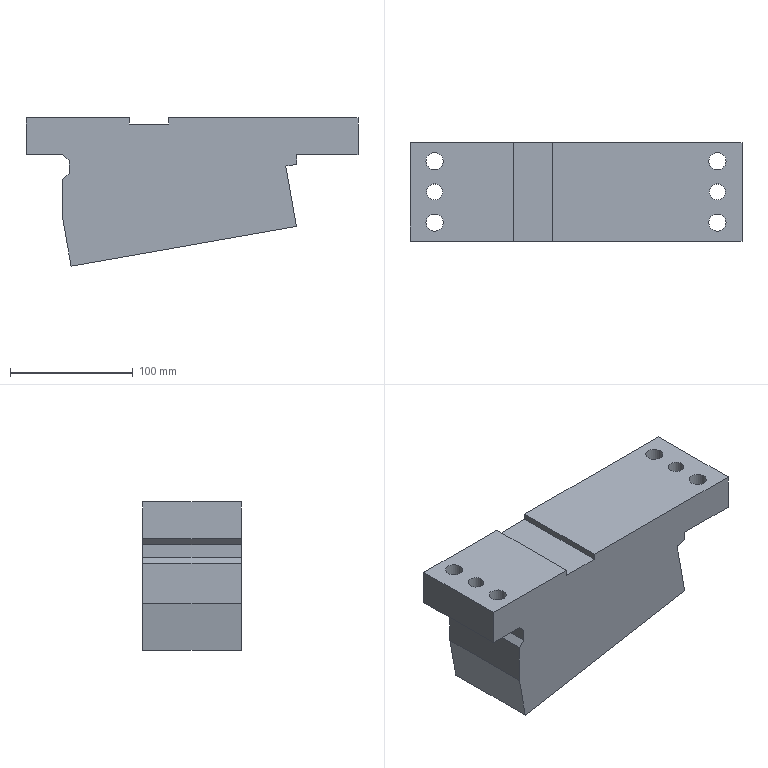Part | NX | features solid 2 | 1 solid | 34 faces | box 270 x 80 x 120.582 mm | volume 1712817 mm3 | plane 24 | cylinder 10 | commonest cylinder face diameters 14 x4 20 x4 13 x2
STEP:
#1=CARTESIAN_POINT('',(686.661,175.,109.418));
#2=VERTEX_POINT('',#1);
#3=CARTESIAN_POINT('',(869.932,175.,141.734));
#4=VERTEX_POINT('',#3);
#5=CARTESIAN_POINT('',(894.552,175.,146.075));
#6=DIRECTION('',(0.9848,0.,0.1736));
#7=VECTOR('',#6,1000.);
#8=LINE('',#5,#7);
#9=EDGE_CURVE('',#2,#4,#8,.T.);
#10=ORIENTED_EDGE('',*,*,#9,.F.);
#11=CARTESIAN_POINT('',(686.661,255.,109.418));
#12=VERTEX_POINT('',#11);
#13=CARTESIAN_POINT('',(686.661,215.,109.418));
#14=DIRECTION('',(0.,1.,0.));
#15=VECTOR('',#14,1000.);
#16=LINE('',#13,#15);
#17=EDGE_CURVE('',#2,#12,#16,.T.);
#18=ORIENTED_EDGE('',*,*,#17,.T.);
#19=CARTESIAN_POINT('',(869.932,255.,141.734));
#20=VERTEX_POINT('',#19);
#21=CARTESIAN_POINT('',(794.948,255.,128.512));
#22=DIRECTION('',(-0.9848,0.,-0.1736));
#23=VECTOR('',#22,1000.);
#24=LINE('',#21,#23);
#25=EDGE_CURVE('',#20,#12,#24,.T.);
#26=ORIENTED_EDGE('',*,*,#25,.F.);
#27=CARTESIAN_POINT('',(869.932,215.,141.734));
#28=DIRECTION('',(0.,1.,0.));
#29=VECTOR('',#28,1000.);
#30=LINE('',#27,#29);
#31=EDGE_CURVE('',#4,#20,#30,.T.);
#32=ORIENTED_EDGE('',*,*,#31,.F.);
#33=EDGE_LOOP('',(#10,#18,#26,#32));
#34=FACE_BOUND('',#33,.T.);
#35=CARTESIAN_POINT('',(894.552,215.,146.075));
#36=DIRECTION('',(0.1736,0.,-0.9848));
#37=DIRECTION('',(0.9848,0.,0.1736));
#38=AXIS2_PLACEMENT_3D('',#35,#36,#37);
#39=PLANE('',#38);
#40=ADVANCED_FACE('',(#34),#39,.T.);
#41=CARTESIAN_POINT('',(680.,255.,147.192));
#42=VERTEX_POINT('',#41);
#43=CARTESIAN_POINT('',(676.242,255.,168.507));
#44=DIRECTION('',(0.1736,0.,-0.9848));
#45=VECTOR('',#44,1000.);
#46=LINE('',#43,#45);
#47=EDGE_CURVE('',#42,#12,#46,.T.);
#48=ORIENTED_EDGE('',*,*,#47,.F.);
#49=CARTESIAN_POINT('',(680.,255.,180.));
#50=VERTEX_POINT('',#49);
#51=CARTESIAN_POINT('',(680.,255.,180.));
#52=DIRECTION('',(0.,0.,-1.));
#53=VECTOR('',#52,1000.);
#54=LINE('',#51,#53);
#55=EDGE_CURVE('',#50,#42,#54,.T.);
#56=ORIENTED_EDGE('',*,*,#55,.F.);
#57=CARTESIAN_POINT('',(685.,255.,185.));
#58=VERTEX_POINT('',#57);
#59=CARTESIAN_POINT('',(680.,255.,180.));
#60=DIRECTION('',(-0.7071,0.,-0.7071));
#61=VECTOR('',#60,1000.);
#62=LINE('',#59,#61);
#63=EDGE_CURVE('',#50,#58,#62,.F.);
#64=ORIENTED_EDGE('',*,*,#63,.T.);
#65=CARTESIAN_POINT('',(685.,255.,195.));
#66=VERTEX_POINT('',#65);
#67=CARTESIAN_POINT('',(685.,255.,145.));
#68=DIRECTION('',(0.,0.,1.));
#69=VECTOR('',#68,1000.);
#70=LINE('',#67,#69);
#71=EDGE_CURVE('',#58,#66,#70,.T.);
#72=ORIENTED_EDGE('',*,*,#71,.T.);
#73=CARTESIAN_POINT('',(680.,255.,200.));
#74=VERTEX_POINT('',#73);
#75=CARTESIAN_POINT('',(685.,255.,195.));
#76=DIRECTION('',(-0.7071,0.,0.7071));
#77=VECTOR('',#76,1000.);
#78=LINE('',#75,#77);
#79=EDGE_CURVE('',#66,#74,#78,.T.);
#80=ORIENTED_EDGE('',*,*,#79,.T.);
#81=CARTESIAN_POINT('',(650.,255.,200.));
#82=VERTEX_POINT('',#81);
#83=CARTESIAN_POINT('',(650.,255.,200.));
#84=DIRECTION('',(1.,0.,0.));
#85=VECTOR('',#84,1000.);
#86=LINE('',#83,#85);
#87=EDGE_CURVE('',#82,#74,#86,.T.);
#88=ORIENTED_EDGE('',*,*,#87,.F.);
#89=CARTESIAN_POINT('',(650.,255.,230.));
#90=VERTEX_POINT('',#89);
#91=CARTESIAN_POINT('',(650.,255.,230.));
#92=DIRECTION('',(0.,0.,-1.));
#93=VECTOR('',#92,1000.);
#94=LINE('',#91,#93);
#95=EDGE_CURVE('',#90,#82,#94,.T.);
#96=ORIENTED_EDGE('',*,*,#95,.F.);
#97=CARTESIAN_POINT('',(730.,255.,230.));
#98=VERTEX_POINT('',#97);
#99=CARTESIAN_POINT('',(920.,255.,230.));
#100=DIRECTION('',(-1.,0.,0.));
#101=VECTOR('',#100,1000.);
#102=LINE('',#99,#101);
#103=EDGE_CURVE('',#98,#90,#102,.T.);
#104=ORIENTED_EDGE('',*,*,#103,.F.);
#105=CARTESIAN_POINT('',(730.,255.,225.));
#106=VERTEX_POINT('',#105);
#107=CARTESIAN_POINT('',(730.,255.,200.));
#108=DIRECTION('',(0.,0.,-1.));
#109=VECTOR('',#108,1000.);
#110=LINE('',#107,#109);
#111=EDGE_CURVE('',#98,#106,#110,.T.);
#112=ORIENTED_EDGE('',*,*,#111,.T.);
#113=ORIENTED_EDGE('',*,*,#111,.F.);
#114=CARTESIAN_POINT('',(734.,255.,230.));
#115=VERTEX_POINT('',#114);
#116=CARTESIAN_POINT('',(920.,255.,230.));
#117=DIRECTION('',(1.,0.,0.));
#118=VECTOR('',#117,1000.);
#119=LINE('',#116,#118);
#120=EDGE_CURVE('',#115,#98,#119,.F.);
#121=ORIENTED_EDGE('',*,*,#120,.F.);
#122=CARTESIAN_POINT('',(734.,255.,225.));
#123=VERTEX_POINT('',#122);
#124=CARTESIAN_POINT('',(734.,255.,128.933));
#125=DIRECTION('',(0.,0.,1.));
#126=VECTOR('',#125,1000.);
#127=LINE('',#124,#126);
#128=EDGE_CURVE('',#115,#123,#127,.F.);
#129=ORIENTED_EDGE('',*,*,#128,.T.);
#130=CARTESIAN_POINT('',(766.,255.,225.));
#131=VERTEX_POINT('',#130);
#132=CARTESIAN_POINT('',(794.874,255.,225.));
#133=DIRECTION('',(-1.,0.,0.));
#134=VECTOR('',#133,1000.);
#135=LINE('',#132,#134);
#136=EDGE_CURVE('',#123,#131,#135,.F.);
#137=ORIENTED_EDGE('',*,*,#136,.T.);
#138=CARTESIAN_POINT('',(766.,255.,230.));
#139=VERTEX_POINT('',#138);
#140=CARTESIAN_POINT('',(766.,255.,128.933));
#141=DIRECTION('',(0.,0.,-1.));
#142=VECTOR('',#141,1000.);
#143=LINE('',#140,#142);
#144=EDGE_CURVE('',#131,#139,#143,.F.);
#145=ORIENTED_EDGE('',*,*,#144,.T.);
#146=CARTESIAN_POINT('',(920.,255.,230.));
#147=VERTEX_POINT('',#146);
#148=CARTESIAN_POINT('',(920.,255.,230.));
#149=DIRECTION('',(1.,0.,0.));
#150=VECTOR('',#149,1000.);
#151=LINE('',#148,#150);
#152=EDGE_CURVE('',#147,#139,#151,.F.);
#153=ORIENTED_EDGE('',*,*,#152,.F.);
#154=CARTESIAN_POINT('',(920.,255.,200.));
#155=VERTEX_POINT('',#154);
#156=CARTESIAN_POINT('',(920.,255.,200.));
#157=DIRECTION('',(0.,0.,1.));
#158=VECTOR('',#157,1000.);
#159=LINE('',#156,#158);
#160=EDGE_CURVE('',#155,#147,#159,.T.);
#161=ORIENTED_EDGE('',*,*,#160,.F.);
#162=CARTESIAN_POINT('',(870.,255.,200.));
#163=VERTEX_POINT('',#162);
#164=CARTESIAN_POINT('',(650.,255.,200.));
#165=DIRECTION('',(1.,0.,0.));
#166=VECTOR('',#165,1000.);
#167=LINE('',#164,#166);
#168=EDGE_CURVE('',#163,#155,#167,.T.);
#169=ORIENTED_EDGE('',*,*,#168,.F.);
#170=CARTESIAN_POINT('',(870.,255.,192.251));
#171=VERTEX_POINT('',#170);
#172=CARTESIAN_POINT('',(870.,255.,128.933));
#173=DIRECTION('',(0.,0.,-1.));
#174=VECTOR('',#173,1000.);
#175=LINE('',#172,#174);
#176=EDGE_CURVE('',#163,#171,#175,.T.);
#177=ORIENTED_EDGE('',*,*,#176,.T.);
#178=CARTESIAN_POINT('',(861.295,255.,190.716));
#179=VERTEX_POINT('',#178);
#180=CARTESIAN_POINT('',(890.946,255.,195.945));
#181=DIRECTION('',(-0.9848,0.,-0.1736));
#182=VECTOR('',#181,1000.);
#183=LINE('',#180,#182);
#184=EDGE_CURVE('',#179,#171,#183,.F.);
#185=ORIENTED_EDGE('',*,*,#184,.F.);
#186=CARTESIAN_POINT('',(855.806,255.,221.848));
#187=DIRECTION('',(0.1736,0.,-0.9848));
#188=VECTOR('',#187,1000.);
#189=LINE('',#186,#188);
#190=EDGE_CURVE('',#179,#20,#189,.T.);
#191=ORIENTED_EDGE('',*,*,#190,.T.);
#192=ORIENTED_EDGE('',*,*,#25,.T.);
#193=EDGE_LOOP('',(#48,#56,#64,#72,#80,#88,#96,#104,#112,#113,#121,#129,#137,#145,#153,#161,#169,#177,#185,#191,#192));
#194=FACE_BOUND('',#193,.T.);
#195=CARTESIAN_POINT('',(794.874,255.,128.933));
#196=DIRECTION('',(0.,1.,0.));
#197=DIRECTION('',(0.,0.,-1.));
#198=AXIS2_PLACEMENT_3D('',#195,#196,#197);
#199=PLANE('',#198);
#200=ADVANCED_FACE('',(#194),#199,.T.);
#201=CARTESIAN_POINT('',(870.,175.,192.251));
#202=VERTEX_POINT('',#201);
#203=CARTESIAN_POINT('',(870.,175.,200.));
#204=VERTEX_POINT('',#203);
#205=CARTESIAN_POINT('',(870.,175.,200.));
#206=DIRECTION('',(0.,0.,1.));
#207=VECTOR('',#206,1000.);
#208=LINE('',#205,#207);
#209=EDGE_CURVE('',#202,#204,#208,.T.);
#210=ORIENTED_EDGE('',*,*,#209,.F.);
#211=CARTESIAN_POINT('',(870.,215.,192.251));
#212=DIRECTION('',(0.,1.,0.));
#213=VECTOR('',#212,1000.);
#214=LINE('',#211,#213);
#215=EDGE_CURVE('',#171,#202,#214,.F.);
#216=ORIENTED_EDGE('',*,*,#215,.F.);
#217=ORIENTED_EDGE('',*,*,#176,.F.);
#218=CARTESIAN_POINT('',(870.,215.,200.));
#219=DIRECTION('',(0.,1.,0.));
#220=VECTOR('',#219,1000.);
#221=LINE('',#218,#220);
#222=EDGE_CURVE('',#204,#163,#221,.T.);
#223=ORIENTED_EDGE('',*,*,#222,.F.);
#224=EDGE_LOOP('',(#210,#216,#217,#223));
#225=FACE_BOUND('',#224,.T.);
#226=CARTESIAN_POINT('',(870.,215.,200.));
#227=DIRECTION('',(1.,0.,0.));
#228=DIRECTION('',(0.,0.,1.));
#229=AXIS2_PLACEMENT_3D('',#226,#227,#228);
#230=PLANE('',#229);
#231=ADVANCED_FACE('',(#225),#230,.T.);
#232=CARTESIAN_POINT('',(861.295,175.,190.716));
#233=VERTEX_POINT('',#232);
#234=CARTESIAN_POINT('',(890.946,175.,195.945));
#235=DIRECTION('',(-0.9848,0.,-0.1736));
#236=VECTOR('',#235,1000.);
#237=LINE('',#234,#236);
#238=EDGE_CURVE('',#233,#202,#237,.F.);
#239=ORIENTED_EDGE('',*,*,#238,.F.);
#240=CARTESIAN_POINT('',(861.295,215.,190.716));
#241=DIRECTION('',(0.,-1.,0.));
#242=VECTOR('',#241,1000.);
#243=LINE('',#240,#242);
#244=EDGE_CURVE('',#233,#179,#243,.F.);
#245=ORIENTED_EDGE('',*,*,#244,.T.);
#246=ORIENTED_EDGE('',*,*,#184,.T.);
#247=ORIENTED_EDGE('',*,*,#215,.T.);
#248=EDGE_LOOP('',(#239,#245,#246,#247));
#249=FACE_BOUND('',#248,.T.);
#250=CARTESIAN_POINT('',(890.946,215.,195.945));
#251=DIRECTION('',(-0.1736,0.,0.9848));
#252=DIRECTION('',(0.,1.,0.));
#253=AXIS2_PLACEMENT_3D('',#250,#251,#252);
#254=PLANE('',#253);
#255=ADVANCED_FACE('',(#249),#254,.F.);
#256=CARTESIAN_POINT('',(893.5,215.,200.));
#257=VERTEX_POINT('',#256);
#258=CARTESIAN_POINT('',(900.,215.,200.));
#259=DIRECTION('',(0.,0.,1.));
#260=DIRECTION('',(-1.,0.,0.));
#261=AXIS2_PLACEMENT_3D('',#258,#259,#260);
#262=CIRCLE('',#261,6.5);
#263=EDGE_CURVE('',#257,#257,#262,.T.);
#264=ORIENTED_EDGE('',*,*,#263,.T.);
#265=EDGE_LOOP('',(#264));
#266=FACE_BOUND('',#265,.T.);
#267=CARTESIAN_POINT('',(890.,240.,200.));
#268=VERTEX_POINT('',#267);
#269=CARTESIAN_POINT('',(900.,240.,200.));
#270=DIRECTION('',(0.,0.,1.));
#271=DIRECTION('',(-1.,0.,0.));
#272=AXIS2_PLACEMENT_3D('',#269,#270,#271);
#273=CIRCLE('',#272,10.);
#274=EDGE_CURVE('',#268,#268,#273,.T.);
#275=ORIENTED_EDGE('',*,*,#274,.T.);
#276=EDGE_LOOP('',(#275));
#277=FACE_BOUND('',#276,.T.);
#278=CARTESIAN_POINT('',(890.,190.,200.));
#279=VERTEX_POINT('',#278);
#280=CARTESIAN_POINT('',(900.,190.,200.));
#281=DIRECTION('',(0.,0.,-1.));
#282=DIRECTION('',(-1.,0.,0.));
#283=AXIS2_PLACEMENT_3D('',#280,#281,#282);
#284=CIRCLE('',#283,10.);
#285=EDGE_CURVE('',#279,#279,#284,.T.);
#286=ORIENTED_EDGE('',*,*,#285,.F.);
#287=EDGE_LOOP('',(#286));
#288=FACE_BOUND('',#287,.T.);
#289=CARTESIAN_POINT('',(920.,175.,200.));
#290=VERTEX_POINT('',#289);
#291=CARTESIAN_POINT('',(920.,215.,200.));
#292=DIRECTION('',(0.,1.,0.));
#293=VECTOR('',#292,1000.);
#294=LINE('',#291,#293);
#295=EDGE_CURVE('',#290,#155,#294,.T.);
#296=ORIENTED_EDGE('',*,*,#295,.F.);
#297=CARTESIAN_POINT('',(650.,175.,200.));
#298=DIRECTION('',(-1.,0.,0.));
#299=VECTOR('',#298,1000.);
#300=LINE('',#297,#299);
#301=EDGE_CURVE('',#290,#204,#300,.T.);
#302=ORIENTED_EDGE('',*,*,#301,.T.);
#303=ORIENTED_EDGE('',*,*,#222,.T.);
#304=ORIENTED_EDGE('',*,*,#168,.T.);
#305=EDGE_LOOP('',(#296,#302,#303,#304));
#306=FACE_BOUND('',#305,.T.);
#307=CARTESIAN_POINT('',(650.,215.,200.));
#308=DIRECTION('',(0.,0.,1.));
#309=DIRECTION('',(-1.,0.,0.));
#310=AXIS2_PLACEMENT_3D('',#307,#308,#309);
#311=PLANE('',#310);
#312=ADVANCED_FACE('',(#266,#277,#288,#306),#311,.F.);
#313=CARTESIAN_POINT('',(685.,175.,195.));
#314=VERTEX_POINT('',#313);
#315=CARTESIAN_POINT('',(685.,175.,185.));
#316=VERTEX_POINT('',#315);
#317=CARTESIAN_POINT('',(685.,175.,145.));
#318=DIRECTION('',(0.,0.,-1.));
#319=VECTOR('',#318,1000.);
#320=LINE('',#317,#319);
#321=EDGE_CURVE('',#314,#316,#320,.T.);
#322=ORIENTED_EDGE('',*,*,#321,.F.);
#323=CARTESIAN_POINT('',(685.,215.,195.));
#324=DIRECTION('',(0.,1.,0.));
#325=VECTOR('',#324,1000.);
#326=LINE('',#323,#325);
#327=EDGE_CURVE('',#314,#66,#326,.T.);
#328=ORIENTED_EDGE('',*,*,#327,.T.);
#329=ORIENTED_EDGE('',*,*,#71,.F.);
#330=CARTESIAN_POINT('',(685.,215.,185.));
#331=DIRECTION('',(0.,-1.,0.));
#332=VECTOR('',#331,1000.);
#333=LINE('',#330,#332);
#334=EDGE_CURVE('',#58,#316,#333,.T.);
#335=ORIENTED_EDGE('',*,*,#334,.T.);
#336=EDGE_LOOP('',(#322,#328,#329,#335));
#337=FACE_BOUND('',#336,.T.);
#338=CARTESIAN_POINT('',(685.,215.,145.));
#339=DIRECTION('',(-1.,0.,0.));
#340=DIRECTION('',(0.,0.,-1.));
#341=AXIS2_PLACEMENT_3D('',#338,#339,#340);
#342=PLANE('',#341);
#343=ADVANCED_FACE('',(#337),#342,.T.);
#344=ORIENTED_EDGE('',*,*,#244,.F.);
#345=CARTESIAN_POINT('',(855.806,175.,221.848));
#346=DIRECTION('',(0.1736,0.,-0.9848));
#347=VECTOR('',#346,1000.);
#348=LINE('',#345,#347);
#349=EDGE_CURVE('',#233,#4,#348,.T.);
#350=ORIENTED_EDGE('',*,*,#349,.T.);
#351=ORIENTED_EDGE('',*,*,#31,.T.);
#352=ORIENTED_EDGE('',*,*,#190,.F.);
#353=EDGE_LOOP('',(#344,#350,#351,#352));
#354=FACE_BOUND('',#353,.T.);
#355=CARTESIAN_POINT('',(855.806,215.,221.848));
#356=DIRECTION('',(-0.9848,0.,-0.1736));
#357=DIRECTION('',(0.1736,0.,-0.9848));
#358=AXIS2_PLACEMENT_3D('',#355,#356,#357);
#359=PLANE('',#358);
#360=ADVANCED_FACE('',(#354),#359,.F.);
#361=CARTESIAN_POINT('',(676.5,215.,230.));
#362=VERTEX_POINT('',#361);
#363=CARTESIAN_POINT('',(670.,215.,230.));
#364=DIRECTION('',(0.,0.,-1.));
#365=DIRECTION('',(1.,0.,0.));
#366=AXIS2_PLACEMENT_3D('',#363,#364,#365);
#367=CIRCLE('',#366,6.5);
#368=EDGE_CURVE('',#362,#362,#367,.T.);
#369=ORIENTED_EDGE('',*,*,#368,.T.);
#370=EDGE_LOOP('',(#369));
#371=FACE_BOUND('',#370,.T.);
#372=CARTESIAN_POINT('',(677.,240.,230.));
#373=VERTEX_POINT('',#372);
#374=CARTESIAN_POINT('',(670.,240.,230.));
#375=DIRECTION('',(0.,0.,-1.));
#376=DIRECTION('',(1.,0.,0.));
#377=AXIS2_PLACEMENT_3D('',#374,#375,#376);
#378=CIRCLE('',#377,7.);
#379=EDGE_CURVE('',#373,#373,#378,.T.);
#380=ORIENTED_EDGE('',*,*,#379,.T.);
#381=EDGE_LOOP('',(#380));
#382=FACE_BOUND('',#381,.T.);
#383=CARTESIAN_POINT('',(650.,175.,230.));
#384=VERTEX_POINT('',#383);
#385=CARTESIAN_POINT('',(650.,215.,230.));
#386=DIRECTION('',(0.,1.,0.));
#387=VECTOR('',#386,1000.);
#388=LINE('',#385,#387);
#389=EDGE_CURVE('',#384,#90,#388,.T.);
#390=ORIENTED_EDGE('',*,*,#389,.F.);
#391=CARTESIAN_POINT('',(734.,175.,230.));
#392=VERTEX_POINT('',#391);
#393=CARTESIAN_POINT('',(920.,175.,230.));
#394=DIRECTION('',(1.,0.,0.));
#395=VECTOR('',#394,1000.);
#396=LINE('',#393,#395);
#397=EDGE_CURVE('',#384,#392,#396,.T.);
#398=ORIENTED_EDGE('',*,*,#397,.T.);
#399=CARTESIAN_POINT('',(734.,274.586,230.));
#400=DIRECTION('',(0.,-1.,0.));
#401=VECTOR('',#400,1000.);
#402=LINE('',#399,#401);
#403=EDGE_CURVE('',#115,#392,#402,.T.);
#404=ORIENTED_EDGE('',*,*,#403,.F.);
#405=ORIENTED_EDGE('',*,*,#120,.T.);
#406=ORIENTED_EDGE('',*,*,#103,.T.);
#407=EDGE_LOOP('',(#390,#398,#404,#405,#406));
#408=FACE_BOUND('',#407,.T.);
#409=CARTESIAN_POINT('',(677.,190.,230.));
#410=VERTEX_POINT('',#409);
#411=CARTESIAN_POINT('',(670.,190.,230.));
#412=DIRECTION('',(0.,0.,1.));
#413=DIRECTION('',(1.,0.,0.));
#414=AXIS2_PLACEMENT_3D('',#411,#412,#413);
#415=CIRCLE('',#414,7.);
#416=EDGE_CURVE('',#410,#410,#415,.T.);
#417=ORIENTED_EDGE('',*,*,#416,.F.);
#418=EDGE_LOOP('',(#417));
#419=FACE_BOUND('',#418,.T.);
#420=CARTESIAN_POINT('',(920.,215.,230.));
#421=DIRECTION('',(0.,0.,-1.));
#422=DIRECTION('',(1.,0.,0.));
#423=AXIS2_PLACEMENT_3D('',#420,#421,#422);
#424=PLANE('',#423);
#425=ADVANCED_FACE('',(#371,#382,#408,#419),#424,.F.);
#426=CARTESIAN_POINT('',(920.,175.,230.));
#427=VERTEX_POINT('',#426);
#428=CARTESIAN_POINT('',(920.,215.,230.));
#429=DIRECTION('',(0.,1.,0.));
#430=VECTOR('',#429,1000.);
#431=LINE('',#428,#430);
#432=EDGE_CURVE('',#427,#147,#431,.T.);
#433=ORIENTED_EDGE('',*,*,#432,.F.);
#434=CARTESIAN_POINT('',(920.,175.,200.));
#435=DIRECTION('',(0.,0.,-1.));
#436=VECTOR('',#435,1000.);
#437=LINE('',#434,#436);
#438=EDGE_CURVE('',#427,#290,#437,.T.);
#439=ORIENTED_EDGE('',*,*,#438,.T.);
#440=ORIENTED_EDGE('',*,*,#295,.T.);
#441=ORIENTED_EDGE('',*,*,#160,.T.);
#442=EDGE_LOOP('',(#433,#439,#440,#441));
#443=FACE_BOUND('',#442,.T.);
#444=CARTESIAN_POINT('',(920.,215.,200.));
#445=DIRECTION('',(-1.,0.,0.));
#446=DIRECTION('',(0.,0.,-1.));
#447=AXIS2_PLACEMENT_3D('',#444,#445,#446);
#448=PLANE('',#447);
#449=ADVANCED_FACE('',(#443),#448,.F.);
#450=CARTESIAN_POINT('',(906.5,215.,230.));
#451=VERTEX_POINT('',#450);
#452=CARTESIAN_POINT('',(900.,215.,230.));
#453=DIRECTION('',(0.,0.,-1.));
#454=DIRECTION('',(1.,0.,0.));
#455=AXIS2_PLACEMENT_3D('',#452,#453,#454);
#456=CIRCLE('',#455,6.5);
#457=EDGE_CURVE('',#451,#451,#456,.T.);
#458=ORIENTED_EDGE('',*,*,#457,.T.);
#459=EDGE_LOOP('',(#458));
#460=FACE_BOUND('',#459,.T.);
#461=CARTESIAN_POINT('',(907.,240.,230.));
#462=VERTEX_POINT('',#461);
#463=CARTESIAN_POINT('',(900.,240.,230.));
#464=DIRECTION('',(0.,0.,-1.));
#465=DIRECTION('',(1.,0.,0.));
#466=AXIS2_PLACEMENT_3D('',#463,#464,#465);
#467=CIRCLE('',#466,7.);
#468=EDGE_CURVE('',#462,#462,#467,.T.);
#469=ORIENTED_EDGE('',*,*,#468,.T.);
#470=EDGE_LOOP('',(#469));
#471=FACE_BOUND('',#470,.T.);
#472=CARTESIAN_POINT('',(766.,175.,230.));
#473=VERTEX_POINT('',#472);
#474=CARTESIAN_POINT('',(766.,215.,230.));
#475=DIRECTION('',(0.,-1.,0.));
#476=VECTOR('',#475,1000.);
#477=LINE('',#474,#476);
#478=EDGE_CURVE('',#139,#473,#477,.T.);
#479=ORIENTED_EDGE('',*,*,#478,.T.);
#480=CARTESIAN_POINT('',(920.,175.,230.));
#481=DIRECTION('',(1.,0.,0.));
#482=VECTOR('',#481,1000.);
#483=LINE('',#480,#482);
#484=EDGE_CURVE('',#473,#427,#483,.T.);
#485=ORIENTED_EDGE('',*,*,#484,.T.);
#486=ORIENTED_EDGE('',*,*,#432,.T.);
#487=ORIENTED_EDGE('',*,*,#152,.T.);
#488=EDGE_LOOP('',(#479,#485,#486,#487));
#489=FACE_BOUND('',#488,.T.);
#490=CARTESIAN_POINT('',(907.,190.,230.));
#491=VERTEX_POINT('',#490);
#492=CARTESIAN_POINT('',(900.,190.,230.));
#493=DIRECTION('',(0.,0.,1.));
#494=DIRECTION('',(1.,0.,0.));
#495=AXIS2_PLACEMENT_3D('',#492,#493,#494);
#496=CIRCLE('',#495,7.);
#497=EDGE_CURVE('',#491,#491,#496,.T.);
#498=ORIENTED_EDGE('',*,*,#497,.F.);
#499=EDGE_LOOP('',(#498));
#500=FACE_BOUND('',#499,.T.);
#501=CARTESIAN_POINT('',(920.,215.,230.));
#502=DIRECTION('',(0.,0.,-1.));
#503=DIRECTION('',(1.,0.,0.));
#504=AXIS2_PLACEMENT_3D('',#501,#502,#503);
#505=PLANE('',#504);
#506=ADVANCED_FACE('',(#460,#471,#489,#500),#505,.F.);
#507=CARTESIAN_POINT('',(650.,175.,200.));
#508=VERTEX_POINT('',#507);
#509=CARTESIAN_POINT('',(650.,215.,200.));
#510=DIRECTION('',(0.,1.,0.));
#511=VECTOR('',#510,1000.);
#512=LINE('',#509,#511);
#513=EDGE_CURVE('',#508,#82,#512,.T.);
#514=ORIENTED_EDGE('',*,*,#513,.F.);
#515=CARTESIAN_POINT('',(650.,175.,230.));
#516=DIRECTION('',(0.,0.,1.));
#517=VECTOR('',#516,1000.);
#518=LINE('',#515,#517);
#519=EDGE_CURVE('',#508,#384,#518,.T.);
#520=ORIENTED_EDGE('',*,*,#519,.T.);
#521=ORIENTED_EDGE('',*,*,#389,.T.);
#522=ORIENTED_EDGE('',*,*,#95,.T.);
#523=EDGE_LOOP('',(#514,#520,#521,#522));
#524=FACE_BOUND('',#523,.T.);
#525=CARTESIAN_POINT('',(650.,215.,230.));
#526=DIRECTION('',(1.,0.,0.));
#527=DIRECTION('',(0.,0.,1.));
#528=AXIS2_PLACEMENT_3D('',#525,#526,#527);
#529=PLANE('',#528);
#530=ADVANCED_FACE('',(#524),#529,.F.);
#531=CARTESIAN_POINT('',(663.5,215.,200.));
#532=VERTEX_POINT('',#531);
#533=CARTESIAN_POINT('',(670.,215.,200.));
#534=DIRECTION('',(0.,0.,1.));
#535=DIRECTION('',(-1.,0.,0.));
#536=AXIS2_PLACEMENT_3D('',#533,#534,#535);
#537=CIRCLE('',#536,6.5);
#538=EDGE_CURVE('',#532,#532,#537,.T.);
#539=ORIENTED_EDGE('',*,*,#538,.T.);
#540=EDGE_LOOP('',(#539));
#541=FACE_BOUND('',#540,.T.);
#542=CARTESIAN_POINT('',(680.,190.,200.));
#543=VERTEX_POINT('',#542);
#544=CARTESIAN_POINT('',(680.,175.,200.));
#545=VERTEX_POINT('',#544);
#546=CARTESIAN_POINT('',(680.,215.,200.));
#547=DIRECTION('',(0.,-1.,0.));
#548=VECTOR('',#547,1000.);
#549=LINE('',#546,#548);
#550=EDGE_CURVE('',#543,#545,#549,.T.);
#551=ORIENTED_EDGE('',*,*,#550,.T.);
#552=CARTESIAN_POINT('',(650.,175.,200.));
#553=DIRECTION('',(-1.,0.,0.));
#554=VECTOR('',#553,1000.);
#555=LINE('',#552,#554);
#556=EDGE_CURVE('',#545,#508,#555,.T.);
#557=ORIENTED_EDGE('',*,*,#556,.T.);
#558=ORIENTED_EDGE('',*,*,#513,.T.);
#559=ORIENTED_EDGE('',*,*,#87,.T.);
#560=CARTESIAN_POINT('',(680.,240.,200.));
#561=VERTEX_POINT('',#560);
#562=CARTESIAN_POINT('',(680.,215.,200.));
#563=DIRECTION('',(0.,-1.,0.));
#564=VECTOR('',#563,1000.);
#565=LINE('',#562,#564);
#566=EDGE_CURVE('',#74,#561,#565,.T.);
#567=ORIENTED_EDGE('',*,*,#566,.T.);
#568=CARTESIAN_POINT('',(670.,240.,200.));
#569=DIRECTION('',(0.,0.,1.));
#570=DIRECTION('',(-1.,0.,0.));
#571=AXIS2_PLACEMENT_3D('',#568,#569,#570);
#572=CIRCLE('',#571,10.);
#573=EDGE_CURVE('',#561,#561,#572,.T.);
#574=ORIENTED_EDGE('',*,*,#573,.T.);
#575=CARTESIAN_POINT('',(680.,215.,200.));
#576=DIRECTION('',(0.,-1.,0.));
#577=VECTOR('',#576,1000.);
#578=LINE('',#575,#577);
#579=EDGE_CURVE('',#561,#543,#578,.T.);
#580=ORIENTED_EDGE('',*,*,#579,.T.);
#581=CARTESIAN_POINT('',(670.,190.,200.));
#582=DIRECTION('',(0.,0.,-1.));
#583=DIRECTION('',(-1.,0.,0.));
#584=AXIS2_PLACEMENT_3D('',#581,#582,#583);
#585=CIRCLE('',#584,10.);
#586=EDGE_CURVE('',#543,#543,#585,.T.);
#587=ORIENTED_EDGE('',*,*,#586,.F.);
#588=EDGE_LOOP('',(#551,#557,#558,#559,#567,#574,#580,#587));
#589=FACE_BOUND('',#588,.T.);
#590=CARTESIAN_POINT('',(650.,215.,200.));
#591=DIRECTION('',(0.,0.,1.));
#592=DIRECTION('',(-1.,0.,0.));
#593=AXIS2_PLACEMENT_3D('',#590,#591,#592);
#594=PLANE('',#593);
#595=ADVANCED_FACE('',(#541,#589),#594,.F.);
#596=CARTESIAN_POINT('',(663.,240.,203.));
#597=VERTEX_POINT('',#596);
#598=CARTESIAN_POINT('',(670.,240.,203.));
#599=DIRECTION('',(0.,0.,1.));
#600=DIRECTION('',(-1.,0.,0.));
#601=AXIS2_PLACEMENT_3D('',#598,#599,#600);
#602=CIRCLE('',#601,7.);
#603=EDGE_CURVE('',#597,#597,#602,.T.);
#604=ORIENTED_EDGE('',*,*,#603,.F.);
#605=EDGE_LOOP('',(#604));
#606=FACE_BOUND('',#605,.T.);
#607=ORIENTED_EDGE('',*,*,#379,.F.);
#608=EDGE_LOOP('',(#607));
#609=FACE_BOUND('',#608,.T.);
#610=CARTESIAN_POINT('',(670.,240.,250.));
#611=DIRECTION('',(0.,0.,1.));
#612=DIRECTION('',(-1.,0.,0.));
#613=AXIS2_PLACEMENT_3D('',#610,#611,#612);
#614=CYLINDRICAL_SURFACE('',#613,7.);
#615=ADVANCED_FACE('',(#606,#609),#614,.F.);
#616=ORIENTED_EDGE('',*,*,#603,.T.);
#617=EDGE_LOOP('',(#616));
#618=FACE_BOUND('',#617,.T.);
#619=CARTESIAN_POINT('',(660.,240.,203.));
#620=VERTEX_POINT('',#619);
#621=CARTESIAN_POINT('',(670.,240.,203.));
#622=DIRECTION('',(0.,0.,1.));
#623=DIRECTION('',(-1.,0.,0.));
#624=AXIS2_PLACEMENT_3D('',#621,#622,#623);
#625=CIRCLE('',#624,10.);
#626=EDGE_CURVE('',#620,#620,#625,.T.);
#627=ORIENTED_EDGE('',*,*,#626,.F.);
#628=EDGE_LOOP('',(#627));
#629=FACE_BOUND('',#628,.T.);
#630=CARTESIAN_POINT('',(670.,240.,203.));
#631=DIRECTION('',(0.,0.,1.));
#632=DIRECTION('',(-1.,0.,0.));
#633=AXIS2_PLACEMENT_3D('',#630,#631,#632);
#634=PLANE('',#633);
#635=ADVANCED_FACE('',(#618,#629),#634,.F.);
#636=ORIENTED_EDGE('',*,*,#626,.T.);
#637=EDGE_LOOP('',(#636));
#638=FACE_BOUND('',#637,.T.);
#639=ORIENTED_EDGE('',*,*,#573,.F.);
#640=EDGE_LOOP('',(#639));
#641=FACE_BOUND('',#640,.T.);
#642=CARTESIAN_POINT('',(670.,240.,200.));
#643=DIRECTION('',(0.,0.,1.));
#644=DIRECTION('',(-1.,0.,0.));
#645=AXIS2_PLACEMENT_3D('',#642,#643,#644);
#646=CYLINDRICAL_SURFACE('',#645,10.);
#647=ADVANCED_FACE('',(#638,#641),#646,.F.);
#648=CARTESIAN_POINT('',(893.,240.,203.));
#649=VERTEX_POINT('',#648);
#650=CARTESIAN_POINT('',(900.,240.,203.));
#651=DIRECTION('',(0.,0.,1.));
#652=DIRECTION('',(-1.,0.,0.));
#653=AXIS2_PLACEMENT_3D('',#650,#651,#652);
#654=CIRCLE('',#653,7.);
#655=EDGE_CURVE('',#649,#649,#654,.T.);
#656=ORIENTED_EDGE('',*,*,#655,.F.);
#657=EDGE_LOOP('',(#656));
#658=FACE_BOUND('',#657,.T.);
#659=ORIENTED_EDGE('',*,*,#468,.F.);
#660=EDGE_LOOP('',(#659));
#661=FACE_BOUND('',#660,.T.);
#662=CARTESIAN_POINT('',(900.,240.,250.));
#663=DIRECTION('',(0.,0.,1.));
#664=DIRECTION('',(-1.,0.,0.));
#665=AXIS2_PLACEMENT_3D('',#662,#663,#664);
#666=CYLINDRICAL_SURFACE('',#665,7.);
#667=ADVANCED_FACE('',(#658,#661),#666,.F.);
#668=ORIENTED_EDGE('',*,*,#655,.T.);
#669=EDGE_LOOP('',(#668));
#670=FACE_BOUND('',#669,.T.);
#671=CARTESIAN_POINT('',(890.,240.,203.));
#672=VERTEX_POINT('',#671);
#673=CARTESIAN_POINT('',(900.,240.,203.));
#674=DIRECTION('',(0.,0.,1.));
#675=DIRECTION('',(-1.,0.,0.));
#676=AXIS2_PLACEMENT_3D('',#673,#674,#675);
#677=CIRCLE('',#676,10.);
#678=EDGE_CURVE('',#672,#672,#677,.T.);
#679=ORIENTED_EDGE('',*,*,#678,.F.);
#680=EDGE_LOOP('',(#679));
#681=FACE_BOUND('',#680,.T.);
#682=CARTESIAN_POINT('',(900.,240.,203.));
#683=DIRECTION('',(0.,0.,1.));
#684=DIRECTION('',(-1.,0.,0.));
#685=AXIS2_PLACEMENT_3D('',#682,#683,#684);
#686=PLANE('',#685);
#687=ADVANCED_FACE('',(#670,#681),#686,.F.);
#688=ORIENTED_EDGE('',*,*,#678,.T.);
#689=EDGE_LOOP('',(#688));
#690=FACE_BOUND('',#689,.T.);
#691=ORIENTED_EDGE('',*,*,#274,.F.);
#692=EDGE_LOOP('',(#691));
#693=FACE_BOUND('',#692,.T.);
#694=CARTESIAN_POINT('',(900.,240.,200.));
#695=DIRECTION('',(0.,0.,1.));
#696=DIRECTION('',(-1.,0.,0.));
#697=AXIS2_PLACEMENT_3D('',#694,#695,#696);
#698=CYLINDRICAL_SURFACE('',#697,10.);
#699=ADVANCED_FACE('',(#690,#693),#698,.F.);
#700=ORIENTED_EDGE('',*,*,#403,.T.);
#701=CARTESIAN_POINT('',(734.,175.,225.));
#702=VERTEX_POINT('',#701);
#703=CARTESIAN_POINT('',(734.,175.,230.));
#704=DIRECTION('',(0.,0.,-1.));
#705=VECTOR('',#704,1000.);
#706=LINE('',#703,#705);
#707=EDGE_CURVE('',#392,#702,#706,.T.);
#708=ORIENTED_EDGE('',*,*,#707,.T.);
#709=CARTESIAN_POINT('',(734.,274.586,225.));
#710=DIRECTION('',(0.,-1.,0.));
#711=VECTOR('',#710,1000.);
#712=LINE('',#709,#711);
#713=EDGE_CURVE('',#123,#702,#712,.T.);
#714=ORIENTED_EDGE('',*,*,#713,.F.);
#715=ORIENTED_EDGE('',*,*,#128,.F.);
#716=EDGE_LOOP('',(#700,#708,#714,#715));
#717=FACE_BOUND('',#716,.T.);
#718=CARTESIAN_POINT('',(734.,274.586,230.));
#719=DIRECTION('',(-1.,0.,0.));
#720=DIRECTION('',(0.,0.,-1.));
#721=AXIS2_PLACEMENT_3D('',#718,#719,#720);
#722=PLANE('',#721);
#723=ADVANCED_FACE('',(#717),#722,.F.);
#724=ORIENTED_EDGE('',*,*,#713,.T.);
#725=CARTESIAN_POINT('',(766.,175.,225.));
#726=VERTEX_POINT('',#725);
#727=CARTESIAN_POINT('',(786.,175.,225.));
#728=DIRECTION('',(1.,0.,0.));
#729=VECTOR('',#728,1000.);
#730=LINE('',#727,#729);
#731=EDGE_CURVE('',#702,#726,#730,.T.);
#732=ORIENTED_EDGE('',*,*,#731,.T.);
#733=CARTESIAN_POINT('',(766.,274.586,225.));
#734=DIRECTION('',(0.,-1.,0.));
#735=VECTOR('',#734,1000.);
#736=LINE('',#733,#735);
#737=EDGE_CURVE('',#131,#726,#736,.T.);
#738=ORIENTED_EDGE('',*,*,#737,.F.);
#739=ORIENTED_EDGE('',*,*,#136,.F.);
#740=EDGE_LOOP('',(#724,#732,#738,#739));
#741=FACE_BOUND('',#740,.T.);
#742=CARTESIAN_POINT('',(786.,274.586,225.));
#743=DIRECTION('',(0.,0.,-1.));
#744=DIRECTION('',(1.,0.,0.));
#745=AXIS2_PLACEMENT_3D('',#742,#743,#744);
#746=PLANE('',#745);
#747=ADVANCED_FACE('',(#741),#746,.F.);
#748=ORIENTED_EDGE('',*,*,#737,.T.);
#749=CARTESIAN_POINT('',(766.,175.,230.));
#750=DIRECTION('',(0.,0.,1.));
#751=VECTOR('',#750,1000.);
#752=LINE('',#749,#751);
#753=EDGE_CURVE('',#726,#473,#752,.T.);
#754=ORIENTED_EDGE('',*,*,#753,.T.);
#755=ORIENTED_EDGE('',*,*,#478,.F.);
#756=ORIENTED_EDGE('',*,*,#144,.F.);
#757=EDGE_LOOP('',(#748,#754,#755,#756));
#758=FACE_BOUND('',#757,.T.);
#759=CARTESIAN_POINT('',(766.,174.586,230.));
#760=DIRECTION('',(1.,0.,0.));
#761=DIRECTION('',(0.,0.,1.));
#762=AXIS2_PLACEMENT_3D('',#759,#760,#761);
#763=PLANE('',#762);
#764=ADVANCED_FACE('',(#758),#763,.F.);
#765=CARTESIAN_POINT('',(663.,190.,203.));
#766=VERTEX_POINT('',#765);
#767=CARTESIAN_POINT('',(670.,190.,203.));
#768=DIRECTION('',(0.,0.,1.));
#769=DIRECTION('',(-1.,0.,0.));
#770=AXIS2_PLACEMENT_3D('',#767,#768,#769);
#771=CIRCLE('',#770,7.);
#772=EDGE_CURVE('',#766,#766,#771,.F.);
#773=ORIENTED_EDGE('',*,*,#772,.T.);
#774=EDGE_LOOP('',(#773));
#775=FACE_BOUND('',#774,.T.);
#776=ORIENTED_EDGE('',*,*,#416,.T.);
#777=EDGE_LOOP('',(#776));
#778=FACE_BOUND('',#777,.T.);
#779=CARTESIAN_POINT('',(670.,190.,250.));
#780=DIRECTION('',(0.,0.,1.));
#781=DIRECTION('',(-1.,0.,0.));
#782=AXIS2_PLACEMENT_3D('',#779,#780,#781);
#783=CYLINDRICAL_SURFACE('',#782,7.);
#784=ADVANCED_FACE('',(#775,#778),#783,.F.);
#785=ORIENTED_EDGE('',*,*,#772,.F.);
#786=EDGE_LOOP('',(#785));
#787=FACE_BOUND('',#786,.T.);
#788=CARTESIAN_POINT('',(660.,190.,203.));
#789=VERTEX_POINT('',#788);
#790=CARTESIAN_POINT('',(670.,190.,203.));
#791=DIRECTION('',(0.,0.,1.));
#792=DIRECTION('',(-1.,0.,0.));
#793=AXIS2_PLACEMENT_3D('',#790,#791,#792);
#794=CIRCLE('',#793,10.);
#795=EDGE_CURVE('',#789,#789,#794,.F.);
#796=ORIENTED_EDGE('',*,*,#795,.T.);
#797=EDGE_LOOP('',(#796));
#798=FACE_BOUND('',#797,.T.);
#799=CARTESIAN_POINT('',(670.,190.,203.));
#800=DIRECTION('',(0.,0.,1.));
#801=DIRECTION('',(-1.,0.,0.));
#802=AXIS2_PLACEMENT_3D('',#799,#800,#801);
#803=PLANE('',#802);
#804=ADVANCED_FACE('',(#787,#798),#803,.F.);
#805=ORIENTED_EDGE('',*,*,#795,.F.);
#806=EDGE_LOOP('',(#805));
#807=FACE_BOUND('',#806,.T.);
#808=ORIENTED_EDGE('',*,*,#586,.T.);
#809=EDGE_LOOP('',(#808));
#810=FACE_BOUND('',#809,.T.);
#811=CARTESIAN_POINT('',(670.,190.,200.));
#812=DIRECTION('',(0.,0.,1.));
#813=DIRECTION('',(-1.,0.,0.));
#814=AXIS2_PLACEMENT_3D('',#811,#812,#813);
#815=CYLINDRICAL_SURFACE('',#814,10.);
#816=ADVANCED_FACE('',(#807,#810),#815,.F.);
#817=CARTESIAN_POINT('',(893.,190.,203.));
#818=VERTEX_POINT('',#817);
#819=CARTESIAN_POINT('',(900.,190.,203.));
#820=DIRECTION('',(0.,0.,1.));
#821=DIRECTION('',(-1.,0.,0.));
#822=AXIS2_PLACEMENT_3D('',#819,#820,#821);
#823=CIRCLE('',#822,7.);
#824=EDGE_CURVE('',#818,#818,#823,.F.);
#825=ORIENTED_EDGE('',*,*,#824,.T.);
#826=EDGE_LOOP('',(#825));
#827=FACE_BOUND('',#826,.T.);
#828=ORIENTED_EDGE('',*,*,#497,.T.);
#829=EDGE_LOOP('',(#828));
#830=FACE_BOUND('',#829,.T.);
#831=CARTESIAN_POINT('',(900.,190.,250.));
#832=DIRECTION('',(0.,0.,1.));
#833=DIRECTION('',(-1.,0.,0.));
#834=AXIS2_PLACEMENT_3D('',#831,#832,#833);
#835=CYLINDRICAL_SURFACE('',#834,7.);
#836=ADVANCED_FACE('',(#827,#830),#835,.F.);
#837=ORIENTED_EDGE('',*,*,#824,.F.);
#838=EDGE_LOOP('',(#837));
#839=FACE_BOUND('',#838,.T.);
#840=CARTESIAN_POINT('',(890.,190.,203.));
#841=VERTEX_POINT('',#840);
#842=CARTESIAN_POINT('',(900.,190.,203.));
#843=DIRECTION('',(0.,0.,1.));
#844=DIRECTION('',(-1.,0.,0.));
#845=AXIS2_PLACEMENT_3D('',#842,#843,#844);
#846=CIRCLE('',#845,10.);
#847=EDGE_CURVE('',#841,#841,#846,.F.);
#848=ORIENTED_EDGE('',*,*,#847,.T.);
#849=EDGE_LOOP('',(#848));
#850=FACE_BOUND('',#849,.T.);
#851=CARTESIAN_POINT('',(900.,190.,203.));
#852=DIRECTION('',(0.,0.,1.));
#853=DIRECTION('',(-1.,0.,0.));
#854=AXIS2_PLACEMENT_3D('',#851,#852,#853);
#855=PLANE('',#854);
#856=ADVANCED_FACE('',(#839,#850),#855,.F.);
#857=ORIENTED_EDGE('',*,*,#847,.F.);
#858=EDGE_LOOP('',(#857));
#859=FACE_BOUND('',#858,.T.);
#860=ORIENTED_EDGE('',*,*,#285,.T.);
#861=EDGE_LOOP('',(#860));
#862=FACE_BOUND('',#861,.T.);
#863=CARTESIAN_POINT('',(900.,190.,200.));
#864=DIRECTION('',(0.,0.,1.));
#865=DIRECTION('',(-1.,0.,0.));
#866=AXIS2_PLACEMENT_3D('',#863,#864,#865);
#867=CYLINDRICAL_SURFACE('',#866,10.);
#868=ADVANCED_FACE('',(#859,#862),#867,.F.);
#869=CARTESIAN_POINT('',(680.,175.,180.));
#870=VERTEX_POINT('',#869);
#871=CARTESIAN_POINT('',(680.,175.,147.192));
#872=VERTEX_POINT('',#871);
#873=CARTESIAN_POINT('',(680.,175.,180.));
#874=DIRECTION('',(0.,0.,-1.));
#875=VECTOR('',#874,1000.);
#876=LINE('',#873,#875);
#877=EDGE_CURVE('',#870,#872,#876,.T.);
#878=ORIENTED_EDGE('',*,*,#877,.F.);
#879=CARTESIAN_POINT('',(680.,175.,180.));
#880=DIRECTION('',(0.,-1.,0.));
#881=VECTOR('',#880,1000.);
#882=LINE('',#879,#881);
#883=EDGE_CURVE('',#870,#50,#882,.F.);
#884=ORIENTED_EDGE('',*,*,#883,.T.);
#885=ORIENTED_EDGE('',*,*,#55,.T.);
#886=CARTESIAN_POINT('',(680.,175.,147.192));
#887=DIRECTION('',(0.,-1.,0.));
#888=VECTOR('',#887,1000.);
#889=LINE('',#886,#888);
#890=EDGE_CURVE('',#872,#42,#889,.F.);
#891=ORIENTED_EDGE('',*,*,#890,.F.);
#892=EDGE_LOOP('',(#878,#884,#885,#891));
#893=FACE_BOUND('',#892,.T.);
#894=CARTESIAN_POINT('',(680.,175.,180.));
#895=DIRECTION('',(-1.,0.,0.));
#896=DIRECTION('',(0.,0.,-1.));
#897=AXIS2_PLACEMENT_3D('',#894,#895,#896);
#898=PLANE('',#897);
#899=ADVANCED_FACE('',(#893),#898,.T.);
#900=ORIENTED_EDGE('',*,*,#327,.F.);
#901=CARTESIAN_POINT('',(685.,175.,195.));
#902=DIRECTION('',(-0.7071,0.,0.7071));
#903=VECTOR('',#902,1000.);
#904=LINE('',#901,#903);
#905=EDGE_CURVE('',#314,#545,#904,.T.);
#906=ORIENTED_EDGE('',*,*,#905,.T.);
#907=ORIENTED_EDGE('',*,*,#550,.F.);
#908=ORIENTED_EDGE('',*,*,#579,.F.);
#909=ORIENTED_EDGE('',*,*,#566,.F.);
#910=ORIENTED_EDGE('',*,*,#79,.F.);
#911=EDGE_LOOP('',(#900,#906,#907,#908,#909,#910));
#912=FACE_BOUND('',#911,.T.);
#913=CARTESIAN_POINT('',(685.,215.,195.));
#914=DIRECTION('',(0.7071,0.,0.7071));
#915=DIRECTION('',(-0.7071,0.,0.7071));
#916=AXIS2_PLACEMENT_3D('',#913,#914,#915);
#917=PLANE('',#916);
#918=ADVANCED_FACE('',(#912),#917,.F.);
#919=ORIENTED_EDGE('',*,*,#883,.F.);
#920=CARTESIAN_POINT('',(680.,175.,180.));
#921=DIRECTION('',(-0.7071,0.,-0.7071));
#922=VECTOR('',#921,1000.);
#923=LINE('',#920,#922);
#924=EDGE_CURVE('',#870,#316,#923,.F.);
#925=ORIENTED_EDGE('',*,*,#924,.T.);
#926=ORIENTED_EDGE('',*,*,#334,.F.);
#927=ORIENTED_EDGE('',*,*,#63,.F.);
#928=EDGE_LOOP('',(#919,#925,#926,#927));
#929=FACE_BOUND('',#928,.T.);
#930=CARTESIAN_POINT('',(680.,175.,180.));
#931=DIRECTION('',(-0.7071,0.,0.7071));
#932=DIRECTION('',(-0.7071,0.,-0.7071));
#933=AXIS2_PLACEMENT_3D('',#930,#931,#932);
#934=PLANE('',#933);
#935=ADVANCED_FACE('',(#929),#934,.T.);
#936=CARTESIAN_POINT('',(676.242,175.,168.507));
#937=DIRECTION('',(0.1736,0.,-0.9848));
#938=VECTOR('',#937,1000.);
#939=LINE('',#936,#938);
#940=EDGE_CURVE('',#872,#2,#939,.T.);
#941=ORIENTED_EDGE('',*,*,#940,.F.);
#942=ORIENTED_EDGE('',*,*,#890,.T.);
#943=ORIENTED_EDGE('',*,*,#47,.T.);
#944=ORIENTED_EDGE('',*,*,#17,.F.);
#945=EDGE_LOOP('',(#941,#942,#943,#944));
#946=FACE_BOUND('',#945,.T.);
#947=CARTESIAN_POINT('',(676.242,175.,168.507));
#948=DIRECTION('',(-0.9848,0.,-0.1736));
#949=DIRECTION('',(0.1736,0.,-0.9848));
#950=AXIS2_PLACEMENT_3D('',#947,#948,#949);
#951=PLANE('',#950);
#952=ADVANCED_FACE('',(#946),#951,.T.);
#953=ORIENTED_EDGE('',*,*,#753,.F.);
#954=ORIENTED_EDGE('',*,*,#731,.F.);
#955=ORIENTED_EDGE('',*,*,#707,.F.);
#956=ORIENTED_EDGE('',*,*,#397,.F.);
#957=ORIENTED_EDGE('',*,*,#519,.F.);
#958=ORIENTED_EDGE('',*,*,#556,.F.);
#959=ORIENTED_EDGE('',*,*,#905,.F.);
#960=ORIENTED_EDGE('',*,*,#321,.T.);
#961=ORIENTED_EDGE('',*,*,#924,.F.);
#962=ORIENTED_EDGE('',*,*,#877,.T.);
#963=ORIENTED_EDGE('',*,*,#940,.T.);
#964=ORIENTED_EDGE('',*,*,#9,.T.);
#965=ORIENTED_EDGE('',*,*,#349,.F.);
#966=ORIENTED_EDGE('',*,*,#238,.T.);
#967=ORIENTED_EDGE('',*,*,#209,.T.);
#968=ORIENTED_EDGE('',*,*,#301,.F.);
#969=ORIENTED_EDGE('',*,*,#438,.F.);
#970=ORIENTED_EDGE('',*,*,#484,.F.);
#971=EDGE_LOOP('',(#953,#954,#955,#956,#957,#958,#959,#960,#961,#962,#963,#964,#965,#966,#967,#968,#969,#970));
#972=FACE_BOUND('',#971,.T.);
#973=CARTESIAN_POINT('',(885.,175.,-15.));
#974=DIRECTION('',(0.,1.,0.));
#975=DIRECTION('',(0.,0.,-1.));
#976=AXIS2_PLACEMENT_3D('',#973,#974,#975);
#977=PLANE('',#976);
#978=ADVANCED_FACE('',(#972),#977,.F.);
#979=ORIENTED_EDGE('',*,*,#263,.F.);
#980=EDGE_LOOP('',(#979));
#981=FACE_BOUND('',#980,.T.);
#982=ORIENTED_EDGE('',*,*,#457,.F.);
#983=EDGE_LOOP('',(#982));
#984=FACE_BOUND('',#983,.T.);
#985=CARTESIAN_POINT('',(900.,215.,200.));
#986=DIRECTION('',(0.,0.,1.));
#987=DIRECTION('',(-1.,0.,0.));
#988=AXIS2_PLACEMENT_3D('',#985,#986,#987);
#989=CYLINDRICAL_SURFACE('',#988,6.5);
#990=ADVANCED_FACE('',(#981,#984),#989,.F.);
#991=ORIENTED_EDGE('',*,*,#538,.F.);
#992=EDGE_LOOP('',(#991));
#993=FACE_BOUND('',#992,.T.);
#994=ORIENTED_EDGE('',*,*,#368,.F.);
#995=EDGE_LOOP('',(#994));
#996=FACE_BOUND('',#995,.T.);
#997=CARTESIAN_POINT('',(670.,215.,200.));
#998=DIRECTION('',(0.,0.,1.));
#999=DIRECTION('',(-1.,0.,0.));
#1000=AXIS2_PLACEMENT_3D('',#997,#998,#999);
#1001=CYLINDRICAL_SURFACE('',#1000,6.5);
#1002=ADVANCED_FACE('',(#993,#996),#1001,.F.);
#1003=CLOSED_SHELL('',(#40,#200,#231,#255,#312,#343,#360,#425,#449,#506,#530,#595,#615,#635,#647,#667,#687,#699,#723,#747,#764,#784,#804,#816,#836,#856,#868,#899,#918,#935,#952,#978,#990,#1002));
#1004=MANIFOLD_SOLID_BREP('',#1003);
#1005=(LENGTH_UNIT()NAMED_UNIT(*)SI_UNIT(.MILLI.,.METRE.));
#1006=UNCERTAINTY_MEASURE_WITH_UNIT(LENGTH_MEASURE(0.00001),#1005,'','');
#1007=(NAMED_UNIT(*)PLANE_ANGLE_UNIT()SI_UNIT($,.RADIAN.));
#1008=(NAMED_UNIT(*)SI_UNIT($,.STERADIAN.)SOLID_ANGLE_UNIT());
#1009=(GEOMETRIC_REPRESENTATION_CONTEXT(3)GLOBAL_UNCERTAINTY_ASSIGNED_CONTEXT((#1006))GLOBAL_UNIT_ASSIGNED_CONTEXT((#1005,#1007,#1008))REPRESENTATION_CONTEXT('',''));
#1010=ADVANCED_BREP_SHAPE_REPRESENTATION('',(#1004),#1009);